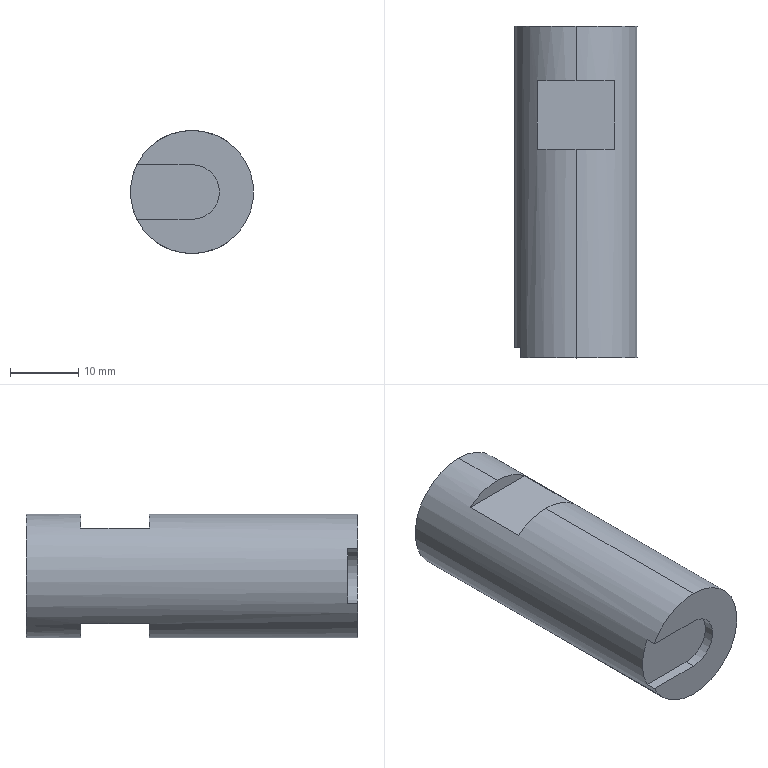Part | STEP file | OP10-150_clamp rod (L) | 1 solid | 18 faces | box 18 x 48.5 x 18 mm | volume 11527 mm3 | plane 11 | cylinder 5 | cone 2 | commonest cylinder face diameters 5 x2 18 x2 8 x1
STEP:
#1=CARTESIAN_POINT('',(0.,0.,0.));
#2=DIRECTION('',(0.,0.,1.));
#3=DIRECTION('',(1.,0.,0.));
#4=AXIS2_PLACEMENT_3D('',#1,#2,#3);
#5=CARTESIAN_POINT('',(0.,30.5,2.5));
#6=VERTEX_POINT('',#5);
#7=CARTESIAN_POINT('',(0.,48.5,2.5));
#8=VERTEX_POINT('',#7);
#9=CARTESIAN_POINT('',(0.,48.5,2.5));
#10=DIRECTION('',(0.,1.,0.));
#11=VECTOR('',#10,1.);
#12=LINE('',#9,#11);
#13=CARTESIAN_POINT('',(0.,48.5,0.));
#14=DIRECTION('',(0.,1.,0.));
#15=DIRECTION('',(0.,0.,1.));
#16=AXIS2_PLACEMENT_3D('',#13,#14,#15);
#17=CYLINDRICAL_SURFACE('',#16,2.5);
#18=CARTESIAN_POINT('',(6.283,0.));
#19=DIRECTION('',(0.,1.));
#20=VECTOR('',#19,1.);
#21=LINE('',#18,#20);
#22=(GEOMETRIC_REPRESENTATION_CONTEXT(2)PARAMETRIC_REPRESENTATION_CONTEXT()REPRESENTATION_CONTEXT('',''));
#23=DEFINITIONAL_REPRESENTATION('',(#21),#22);
#24=PCURVE('',#17,#23);
#25=CARTESIAN_POINT('',(0.,48.5,0.));
#26=DIRECTION('',(0.,1.,0.));
#27=DIRECTION('',(0.,0.,1.));
#28=AXIS2_PLACEMENT_3D('',#25,#26,#27);
#29=CYLINDRICAL_SURFACE('',#28,2.5);
#30=CARTESIAN_POINT('',(0.,0.));
#31=DIRECTION('',(0.,1.));
#32=VECTOR('',#31,1.);
#33=LINE('',#30,#32);
#34=(GEOMETRIC_REPRESENTATION_CONTEXT(2)PARAMETRIC_REPRESENTATION_CONTEXT()REPRESENTATION_CONTEXT('',''));
#35=DEFINITIONAL_REPRESENTATION('',(#33),#34);
#36=PCURVE('',#29,#35);
#37=SURFACE_CURVE('',#12,(#24,#36),.PCURVE_S1.);
#38=EDGE_CURVE('',#6,#8,#37,.T.);
#39=ORIENTED_EDGE('',*,*,#38,.T.);
#40=CARTESIAN_POINT('',(0.,48.5,-2.5));
#41=VERTEX_POINT('',#40);
#42=CARTESIAN_POINT('',(0.,48.5,0.));
#43=DIRECTION('',(0.,1.,0.));
#44=DIRECTION('',(0.,0.,1.));
#45=AXIS2_PLACEMENT_3D('',#42,#43,#44);
#46=CIRCLE('',#45,2.5);
#47=CARTESIAN_POINT('',(0.,0.));
#48=DIRECTION('',(1.,0.));
#49=VECTOR('',#48,1.);
#50=LINE('',#47,#49);
#51=(GEOMETRIC_REPRESENTATION_CONTEXT(2)PARAMETRIC_REPRESENTATION_CONTEXT()REPRESENTATION_CONTEXT('',''));
#52=DEFINITIONAL_REPRESENTATION('',(#50),#51);
#53=PCURVE('',#17,#52);
#54=CARTESIAN_POINT('',(0.,48.5,0.));
#55=DIRECTION('',(0.,1.,0.));
#56=DIRECTION('',(0.,0.,1.));
#57=AXIS2_PLACEMENT_3D('',#54,#55,#56);
#58=PLANE('',#57);
#59=CARTESIAN_POINT('',(0.,0.));
#60=DIRECTION('',(1.,0.));
#61=AXIS2_PLACEMENT_2D('',#59,#60);
#62=CIRCLE('',#61,2.5);
#63=(GEOMETRIC_REPRESENTATION_CONTEXT(2)PARAMETRIC_REPRESENTATION_CONTEXT()REPRESENTATION_CONTEXT('',''));
#64=DEFINITIONAL_REPRESENTATION('',(#62),#63);
#65=PCURVE('',#58,#64);
#66=SURFACE_CURVE('',#46,(#53,#65),.PCURVE_S1.);
#67=EDGE_CURVE('',#41,#8,#66,.T.);
#68=ORIENTED_EDGE('',*,*,#67,.F.);
#69=CARTESIAN_POINT('',(0.,30.5,-2.5));
#70=VERTEX_POINT('',#69);
#71=CARTESIAN_POINT('',(0.,48.5,-2.5));
#72=DIRECTION('',(0.,1.,0.));
#73=VECTOR('',#72,1.);
#74=LINE('',#71,#73);
#75=CARTESIAN_POINT('',(3.142,0.));
#76=DIRECTION('',(0.,1.));
#77=VECTOR('',#76,1.);
#78=LINE('',#75,#77);
#79=(GEOMETRIC_REPRESENTATION_CONTEXT(2)PARAMETRIC_REPRESENTATION_CONTEXT()REPRESENTATION_CONTEXT('',''));
#80=DEFINITIONAL_REPRESENTATION('',(#78),#79);
#81=PCURVE('',#17,#80);
#82=CARTESIAN_POINT('',(3.142,0.));
#83=DIRECTION('',(0.,1.));
#84=VECTOR('',#83,1.);
#85=LINE('',#82,#84);
#86=(GEOMETRIC_REPRESENTATION_CONTEXT(2)PARAMETRIC_REPRESENTATION_CONTEXT()REPRESENTATION_CONTEXT('',''));
#87=DEFINITIONAL_REPRESENTATION('',(#85),#86);
#88=PCURVE('',#29,#87);
#89=SURFACE_CURVE('',#74,(#81,#88),.PCURVE_S1.);
#90=EDGE_CURVE('',#70,#41,#89,.T.);
#91=ORIENTED_EDGE('',*,*,#90,.F.);
#92=CARTESIAN_POINT('',(0.,30.5,0.));
#93=DIRECTION('',(0.,1.,0.));
#94=DIRECTION('',(0.,0.,1.));
#95=AXIS2_PLACEMENT_3D('',#92,#93,#94);
#96=CIRCLE('',#95,2.5);
#97=CARTESIAN_POINT('',(0.,-18.));
#98=DIRECTION('',(1.,0.));
#99=VECTOR('',#98,1.);
#100=LINE('',#97,#99);
#101=(GEOMETRIC_REPRESENTATION_CONTEXT(2)PARAMETRIC_REPRESENTATION_CONTEXT()REPRESENTATION_CONTEXT('',''));
#102=DEFINITIONAL_REPRESENTATION('',(#100),#101);
#103=PCURVE('',#17,#102);
#104=CARTESIAN_POINT('',(0.,30.5,0.));
#105=DIRECTION('',(0.,1.,0.));
#106=DIRECTION('',(0.,0.,1.));
#107=AXIS2_PLACEMENT_3D('',#104,#105,#106);
#108=CONICAL_SURFACE('',#107,2.5,1.03);
#109=CARTESIAN_POINT('',(0.,0.));
#110=DIRECTION('',(1.,0.));
#111=VECTOR('',#110,1.);
#112=LINE('',#109,#111);
#113=(GEOMETRIC_REPRESENTATION_CONTEXT(2)PARAMETRIC_REPRESENTATION_CONTEXT()REPRESENTATION_CONTEXT('',''));
#114=DEFINITIONAL_REPRESENTATION('',(#112),#113);
#115=PCURVE('',#108,#114);
#116=SURFACE_CURVE('',#96,(#103,#115),.PCURVE_S1.);
#117=EDGE_CURVE('',#70,#6,#116,.T.);
#118=ORIENTED_EDGE('',*,*,#117,.T.);
#119=EDGE_LOOP('',(#39,#68,#91,#118));
#120=FACE_BOUND('',#119,.F.);
#121=ADVANCED_FACE('',(#120),#17,.F.);
#122=ORIENTED_EDGE('',*,*,#117,.F.);
#123=CARTESIAN_POINT('',(0.,28.998,0.));
#124=VERTEX_POINT('',#123);
#125=CARTESIAN_POINT('',(0.,30.5,-2.5));
#126=DIRECTION('',(0.,0.515,-0.8572));
#127=VECTOR('',#126,1.);
#128=LINE('',#125,#127);
#129=CARTESIAN_POINT('',(3.142,0.));
#130=DIRECTION('',(0.,1.));
#131=VECTOR('',#130,1.);
#132=LINE('',#129,#131);
#133=(GEOMETRIC_REPRESENTATION_CONTEXT(2)PARAMETRIC_REPRESENTATION_CONTEXT()REPRESENTATION_CONTEXT('',''));
#134=DEFINITIONAL_REPRESENTATION('',(#132),#133);
#135=PCURVE('',#108,#134);
#136=CARTESIAN_POINT('',(0.,30.5,0.));
#137=DIRECTION('',(0.,1.,0.));
#138=DIRECTION('',(0.,0.,1.));
#139=AXIS2_PLACEMENT_3D('',#136,#137,#138);
#140=CONICAL_SURFACE('',#139,2.5,1.03);
#141=CARTESIAN_POINT('',(3.142,0.));
#142=DIRECTION('',(0.,1.));
#143=VECTOR('',#142,1.);
#144=LINE('',#141,#143);
#145=(GEOMETRIC_REPRESENTATION_CONTEXT(2)PARAMETRIC_REPRESENTATION_CONTEXT()REPRESENTATION_CONTEXT('',''));
#146=DEFINITIONAL_REPRESENTATION('',(#144),#145);
#147=PCURVE('',#140,#146);
#148=SURFACE_CURVE('',#128,(#135,#147),.PCURVE_S1.);
#149=EDGE_CURVE('',#124,#70,#148,.T.);
#150=ORIENTED_EDGE('',*,*,#149,.F.);
#151=CARTESIAN_POINT('',(0.,30.5,2.5));
#152=DIRECTION('',(0.,0.515,0.8572));
#153=VECTOR('',#152,1.);
#154=LINE('',#151,#153);
#155=CARTESIAN_POINT('',(6.283,0.));
#156=DIRECTION('',(0.,1.));
#157=VECTOR('',#156,1.);
#158=LINE('',#155,#157);
#159=(GEOMETRIC_REPRESENTATION_CONTEXT(2)PARAMETRIC_REPRESENTATION_CONTEXT()REPRESENTATION_CONTEXT('',''));
#160=DEFINITIONAL_REPRESENTATION('',(#158),#159);
#161=PCURVE('',#108,#160);
#162=CARTESIAN_POINT('',(0.,0.));
#163=DIRECTION('',(0.,1.));
#164=VECTOR('',#163,1.);
#165=LINE('',#162,#164);
#166=(GEOMETRIC_REPRESENTATION_CONTEXT(2)PARAMETRIC_REPRESENTATION_CONTEXT()REPRESENTATION_CONTEXT('',''));
#167=DEFINITIONAL_REPRESENTATION('',(#165),#166);
#168=PCURVE('',#140,#167);
#169=SURFACE_CURVE('',#154,(#161,#168),.PCURVE_S1.);
#170=EDGE_CURVE('',#124,#6,#169,.T.);
#171=ORIENTED_EDGE('',*,*,#170,.T.);
#172=EDGE_LOOP('',(#122,#150,#171));
#173=FACE_BOUND('',#172,.F.);
#174=ADVANCED_FACE('',(#173),#108,.F.);
#175=CARTESIAN_POINT('',(0.,48.5,9.));
#176=VERTEX_POINT('',#175);
#177=CARTESIAN_POINT('',(0.,48.5,-9.));
#178=VERTEX_POINT('',#177);
#179=CARTESIAN_POINT('',(0.,48.5,0.));
#180=DIRECTION('',(0.,1.,0.));
#181=DIRECTION('',(0.,0.,1.));
#182=AXIS2_PLACEMENT_3D('',#179,#180,#181);
#183=CIRCLE('',#182,9.);
#184=CARTESIAN_POINT('',(0.,48.5,0.));
#185=DIRECTION('',(0.,-1.,0.));
#186=DIRECTION('',(0.,0.,-1.));
#187=AXIS2_PLACEMENT_3D('',#184,#185,#186);
#188=CYLINDRICAL_SURFACE('',#187,9.);
#189=CARTESIAN_POINT('',(3.142,0.));
#190=DIRECTION('',(-1.,0.));
#191=VECTOR('',#190,1.);
#192=LINE('',#189,#191);
#193=(GEOMETRIC_REPRESENTATION_CONTEXT(2)PARAMETRIC_REPRESENTATION_CONTEXT()REPRESENTATION_CONTEXT('',''));
#194=DEFINITIONAL_REPRESENTATION('',(#192),#193);
#195=PCURVE('',#188,#194);
#196=CARTESIAN_POINT('',(0.,0.));
#197=DIRECTION('',(1.,0.));
#198=AXIS2_PLACEMENT_2D('',#196,#197);
#199=CIRCLE('',#198,9.);
#200=(GEOMETRIC_REPRESENTATION_CONTEXT(2)PARAMETRIC_REPRESENTATION_CONTEXT()REPRESENTATION_CONTEXT('',''));
#201=DEFINITIONAL_REPRESENTATION('',(#199),#200);
#202=PCURVE('',#58,#201);
#203=SURFACE_CURVE('',#183,(#195,#202),.PCURVE_S1.);
#204=EDGE_CURVE('',#176,#178,#203,.T.);
#205=ORIENTED_EDGE('',*,*,#204,.F.);
#206=CARTESIAN_POINT('',(0.,40.5,9.));
#207=VERTEX_POINT('',#206);
#208=CARTESIAN_POINT('',(0.,48.5,9.));
#209=DIRECTION('',(0.,-1.,0.));
#210=VECTOR('',#209,1.);
#211=LINE('',#208,#210);
#212=CARTESIAN_POINT('',(3.142,0.));
#213=DIRECTION('',(0.,1.));
#214=VECTOR('',#213,1.);
#215=LINE('',#212,#214);
#216=(GEOMETRIC_REPRESENTATION_CONTEXT(2)PARAMETRIC_REPRESENTATION_CONTEXT()REPRESENTATION_CONTEXT('',''));
#217=DEFINITIONAL_REPRESENTATION('',(#215),#216);
#218=PCURVE('',#188,#217);
#219=CARTESIAN_POINT('',(0.,48.5,0.));
#220=DIRECTION('',(0.,-1.,0.));
#221=DIRECTION('',(0.,0.,-1.));
#222=AXIS2_PLACEMENT_3D('',#219,#220,#221);
#223=CYLINDRICAL_SURFACE('',#222,9.);
#224=CARTESIAN_POINT('',(3.142,0.));
#225=DIRECTION('',(0.,1.));
#226=VECTOR('',#225,1.);
#227=LINE('',#224,#226);
#228=(GEOMETRIC_REPRESENTATION_CONTEXT(2)PARAMETRIC_REPRESENTATION_CONTEXT()REPRESENTATION_CONTEXT('',''));
#229=DEFINITIONAL_REPRESENTATION('',(#227),#228);
#230=PCURVE('',#223,#229);
#231=SURFACE_CURVE('',#211,(#218,#230),.PCURVE_S1.);
#232=EDGE_CURVE('',#176,#207,#231,.T.);
#233=ORIENTED_EDGE('',*,*,#232,.T.);
#234=CARTESIAN_POINT('',(5.657,40.5,7.));
#235=VERTEX_POINT('',#234);
#236=CARTESIAN_POINT('',(0.,40.5,0.));
#237=DIRECTION('',(0.,-1.,0.));
#238=DIRECTION('',(0.,0.,-1.));
#239=AXIS2_PLACEMENT_3D('',#236,#237,#238);
#240=CIRCLE('',#239,9.);
#241=CARTESIAN_POINT('',(0.,8.));
#242=DIRECTION('',(1.,0.));
#243=VECTOR('',#242,1.);
#244=LINE('',#241,#243);
#245=(GEOMETRIC_REPRESENTATION_CONTEXT(2)PARAMETRIC_REPRESENTATION_CONTEXT()REPRESENTATION_CONTEXT('',''));
#246=DEFINITIONAL_REPRESENTATION('',(#244),#245);
#247=PCURVE('',#188,#246);
#248=CARTESIAN_POINT('',(-16.827,40.5,55.5));
#249=DIRECTION('',(0.,-1.,0.));
#250=DIRECTION('',(0.,0.,-1.));
#251=AXIS2_PLACEMENT_3D('',#248,#249,#250);
#252=PLANE('',#251);
#253=CARTESIAN_POINT('',(55.5,16.827));
#254=DIRECTION('',(1.,0.));
#255=AXIS2_PLACEMENT_2D('',#253,#254);
#256=CIRCLE('',#255,9.);
#257=(GEOMETRIC_REPRESENTATION_CONTEXT(2)PARAMETRIC_REPRESENTATION_CONTEXT()REPRESENTATION_CONTEXT('',''));
#258=DEFINITIONAL_REPRESENTATION('',(#256),#257);
#259=PCURVE('',#252,#258);
#260=SURFACE_CURVE('',#240,(#247,#259),.PCURVE_S1.);
#261=EDGE_CURVE('',#235,#207,#260,.T.);
#262=ORIENTED_EDGE('',*,*,#261,.F.);
#263=CARTESIAN_POINT('',(5.657,30.5,7.));
#264=VERTEX_POINT('',#263);
#265=CARTESIAN_POINT('',(5.657,48.5,7.));
#266=DIRECTION('',(0.,-1.,0.));
#267=VECTOR('',#266,1.);
#268=LINE('',#265,#267);
#269=CARTESIAN_POINT('',(2.462,0.));
#270=DIRECTION('',(0.,1.));
#271=VECTOR('',#270,1.);
#272=LINE('',#269,#271);
#273=(GEOMETRIC_REPRESENTATION_CONTEXT(2)PARAMETRIC_REPRESENTATION_CONTEXT()REPRESENTATION_CONTEXT('',''));
#274=DEFINITIONAL_REPRESENTATION('',(#272),#273);
#275=PCURVE('',#188,#274);
#276=CARTESIAN_POINT('',(0.,0.,7.));
#277=DIRECTION('',(0.,0.,-1.));
#278=DIRECTION('',(1.,0.,0.));
#279=AXIS2_PLACEMENT_3D('',#276,#277,#278);
#280=PLANE('',#279);
#281=CARTESIAN_POINT('',(5.657,-48.5));
#282=DIRECTION('',(0.,1.));
#283=VECTOR('',#282,1.);
#284=LINE('',#281,#283);
#285=(GEOMETRIC_REPRESENTATION_CONTEXT(2)PARAMETRIC_REPRESENTATION_CONTEXT()REPRESENTATION_CONTEXT('',''));
#286=DEFINITIONAL_REPRESENTATION('',(#284),#285);
#287=PCURVE('',#280,#286);
#288=SURFACE_CURVE('',#268,(#275,#287),.PCURVE_S1.);
#289=EDGE_CURVE('',#235,#264,#288,.T.);
#290=ORIENTED_EDGE('',*,*,#289,.T.);
#291=CARTESIAN_POINT('',(0.,30.5,9.));
#292=VERTEX_POINT('',#291);
#293=CARTESIAN_POINT('',(0.,30.5,0.));
#294=DIRECTION('',(0.,1.,0.));
#295=DIRECTION('',(0.,0.,1.));
#296=AXIS2_PLACEMENT_3D('',#293,#294,#295);
#297=CIRCLE('',#296,9.);
#298=CARTESIAN_POINT('',(3.142,18.));
#299=DIRECTION('',(-1.,0.));
#300=VECTOR('',#299,1.);
#301=LINE('',#298,#300);
#302=(GEOMETRIC_REPRESENTATION_CONTEXT(2)PARAMETRIC_REPRESENTATION_CONTEXT()REPRESENTATION_CONTEXT('',''));
#303=DEFINITIONAL_REPRESENTATION('',(#301),#302);
#304=PCURVE('',#188,#303);
#305=CARTESIAN_POINT('',(-16.827,30.5,55.5));
#306=DIRECTION('',(0.,1.,0.));
#307=DIRECTION('',(0.,0.,1.));
#308=AXIS2_PLACEMENT_3D('',#305,#306,#307);
#309=PLANE('',#308);
#310=CARTESIAN_POINT('',(-55.5,16.827));
#311=DIRECTION('',(1.,0.));
#312=AXIS2_PLACEMENT_2D('',#310,#311);
#313=CIRCLE('',#312,9.);
#314=(GEOMETRIC_REPRESENTATION_CONTEXT(2)PARAMETRIC_REPRESENTATION_CONTEXT()REPRESENTATION_CONTEXT('',''));
#315=DEFINITIONAL_REPRESENTATION('',(#313),#314);
#316=PCURVE('',#309,#315);
#317=SURFACE_CURVE('',#297,(#304,#316),.PCURVE_S1.);
#318=EDGE_CURVE('',#292,#264,#317,.T.);
#319=ORIENTED_EDGE('',*,*,#318,.F.);
#320=CARTESIAN_POINT('',(0.,0.,9.));
#321=VERTEX_POINT('',#320);
#322=CARTESIAN_POINT('',(0.,48.5,9.));
#323=DIRECTION('',(0.,-1.,0.));
#324=VECTOR('',#323,1.);
#325=LINE('',#322,#324);
#326=CARTESIAN_POINT('',(3.142,0.));
#327=DIRECTION('',(0.,1.));
#328=VECTOR('',#327,1.);
#329=LINE('',#326,#328);
#330=(GEOMETRIC_REPRESENTATION_CONTEXT(2)PARAMETRIC_REPRESENTATION_CONTEXT()REPRESENTATION_CONTEXT('',''));
#331=DEFINITIONAL_REPRESENTATION('',(#329),#330);
#332=PCURVE('',#188,#331);
#333=CARTESIAN_POINT('',(3.142,0.));
#334=DIRECTION('',(0.,1.));
#335=VECTOR('',#334,1.);
#336=LINE('',#333,#335);
#337=(GEOMETRIC_REPRESENTATION_CONTEXT(2)PARAMETRIC_REPRESENTATION_CONTEXT()REPRESENTATION_CONTEXT('',''));
#338=DEFINITIONAL_REPRESENTATION('',(#336),#337);
#339=PCURVE('',#223,#338);
#340=SURFACE_CURVE('',#325,(#332,#339),.PCURVE_S1.);
#341=EDGE_CURVE('',#292,#321,#340,.T.);
#342=ORIENTED_EDGE('',*,*,#341,.T.);
#343=CARTESIAN_POINT('',(0.,0.,-9.));
#344=VERTEX_POINT('',#343);
#345=CARTESIAN_POINT('',(0.,0.,0.));
#346=DIRECTION('',(0.,1.,0.));
#347=DIRECTION('',(0.,0.,1.));
#348=AXIS2_PLACEMENT_3D('',#345,#346,#347);
#349=CIRCLE('',#348,9.);
#350=CARTESIAN_POINT('',(3.142,48.5));
#351=DIRECTION('',(-1.,0.));
#352=VECTOR('',#351,1.);
#353=LINE('',#350,#352);
#354=(GEOMETRIC_REPRESENTATION_CONTEXT(2)PARAMETRIC_REPRESENTATION_CONTEXT()REPRESENTATION_CONTEXT('',''));
#355=DEFINITIONAL_REPRESENTATION('',(#353),#354);
#356=PCURVE('',#188,#355);
#357=CARTESIAN_POINT('',(0.,0.,0.));
#358=DIRECTION('',(0.,1.,0.));
#359=DIRECTION('',(0.,0.,1.));
#360=AXIS2_PLACEMENT_3D('',#357,#358,#359);
#361=PLANE('',#360);
#362=CARTESIAN_POINT('',(0.,0.));
#363=DIRECTION('',(1.,0.));
#364=AXIS2_PLACEMENT_2D('',#362,#363);
#365=CIRCLE('',#364,9.);
#366=(GEOMETRIC_REPRESENTATION_CONTEXT(2)PARAMETRIC_REPRESENTATION_CONTEXT()REPRESENTATION_CONTEXT('',''));
#367=DEFINITIONAL_REPRESENTATION('',(#365),#366);
#368=PCURVE('',#361,#367);
#369=SURFACE_CURVE('',#349,(#356,#368),.PCURVE_S1.);
#370=EDGE_CURVE('',#321,#344,#369,.T.);
#371=ORIENTED_EDGE('',*,*,#370,.T.);
#372=CARTESIAN_POINT('',(0.,30.5,-9.));
#373=VERTEX_POINT('',#372);
#374=CARTESIAN_POINT('',(0.,48.5,-9.));
#375=DIRECTION('',(0.,-1.,0.));
#376=VECTOR('',#375,1.);
#377=LINE('',#374,#376);
#378=CARTESIAN_POINT('',(0.,0.));
#379=DIRECTION('',(0.,1.));
#380=VECTOR('',#379,1.);
#381=LINE('',#378,#380);
#382=(GEOMETRIC_REPRESENTATION_CONTEXT(2)PARAMETRIC_REPRESENTATION_CONTEXT()REPRESENTATION_CONTEXT('',''));
#383=DEFINITIONAL_REPRESENTATION('',(#381),#382);
#384=PCURVE('',#188,#383);
#385=CARTESIAN_POINT('',(6.283,0.));
#386=DIRECTION('',(0.,1.));
#387=VECTOR('',#386,1.);
#388=LINE('',#385,#387);
#389=(GEOMETRIC_REPRESENTATION_CONTEXT(2)PARAMETRIC_REPRESENTATION_CONTEXT()REPRESENTATION_CONTEXT('',''));
#390=DEFINITIONAL_REPRESENTATION('',(#388),#389);
#391=PCURVE('',#223,#390);
#392=SURFACE_CURVE('',#377,(#384,#391),.PCURVE_S1.);
#393=EDGE_CURVE('',#373,#344,#392,.T.);
#394=ORIENTED_EDGE('',*,*,#393,.F.);
#395=CARTESIAN_POINT('',(5.657,30.5,-7.));
#396=VERTEX_POINT('',#395);
#397=CARTESIAN_POINT('',(0.,30.5,0.));
#398=DIRECTION('',(0.,-1.,0.));
#399=DIRECTION('',(0.,0.,-1.));
#400=AXIS2_PLACEMENT_3D('',#397,#398,#399);
#401=CIRCLE('',#400,9.);
#402=CARTESIAN_POINT('',(0.,18.));
#403=DIRECTION('',(1.,0.));
#404=VECTOR('',#403,1.);
#405=LINE('',#402,#404);
#406=(GEOMETRIC_REPRESENTATION_CONTEXT(2)PARAMETRIC_REPRESENTATION_CONTEXT()REPRESENTATION_CONTEXT('',''));
#407=DEFINITIONAL_REPRESENTATION('',(#405),#406);
#408=PCURVE('',#188,#407);
#409=CARTESIAN_POINT('',(-16.827,30.5,-55.5));
#410=DIRECTION('',(0.,-1.,0.));
#411=DIRECTION('',(0.,0.,-1.));
#412=AXIS2_PLACEMENT_3D('',#409,#410,#411);
#413=PLANE('',#412);
#414=CARTESIAN_POINT('',(-55.5,16.827));
#415=DIRECTION('',(1.,0.));
#416=AXIS2_PLACEMENT_2D('',#414,#415);
#417=CIRCLE('',#416,9.);
#418=(GEOMETRIC_REPRESENTATION_CONTEXT(2)PARAMETRIC_REPRESENTATION_CONTEXT()REPRESENTATION_CONTEXT('',''));
#419=DEFINITIONAL_REPRESENTATION('',(#417),#418);
#420=PCURVE('',#413,#419);
#421=SURFACE_CURVE('',#401,(#408,#420),.PCURVE_S1.);
#422=EDGE_CURVE('',#373,#396,#421,.T.);
#423=ORIENTED_EDGE('',*,*,#422,.T.);
#424=CARTESIAN_POINT('',(5.657,40.5,-7.));
#425=VERTEX_POINT('',#424);
#426=CARTESIAN_POINT('',(5.657,48.5,-7.));
#427=DIRECTION('',(0.,1.,0.));
#428=VECTOR('',#427,1.);
#429=LINE('',#426,#428);
#430=CARTESIAN_POINT('',(0.6797,0.));
#431=DIRECTION('',(0.,-1.));
#432=VECTOR('',#431,1.);
#433=LINE('',#430,#432);
#434=(GEOMETRIC_REPRESENTATION_CONTEXT(2)PARAMETRIC_REPRESENTATION_CONTEXT()REPRESENTATION_CONTEXT('',''));
#435=DEFINITIONAL_REPRESENTATION('',(#433),#434);
#436=PCURVE('',#188,#435);
#437=CARTESIAN_POINT('',(0.,0.,-7.));
#438=DIRECTION('',(0.,0.,1.));
#439=DIRECTION('',(1.,0.,0.));
#440=AXIS2_PLACEMENT_3D('',#437,#438,#439);
#441=PLANE('',#440);
#442=CARTESIAN_POINT('',(5.657,48.5));
#443=DIRECTION('',(0.,1.));
#444=VECTOR('',#443,1.);
#445=LINE('',#442,#444);
#446=(GEOMETRIC_REPRESENTATION_CONTEXT(2)PARAMETRIC_REPRESENTATION_CONTEXT()REPRESENTATION_CONTEXT('',''));
#447=DEFINITIONAL_REPRESENTATION('',(#445),#446);
#448=PCURVE('',#441,#447);
#449=SURFACE_CURVE('',#429,(#436,#448),.PCURVE_S1.);
#450=EDGE_CURVE('',#396,#425,#449,.T.);
#451=ORIENTED_EDGE('',*,*,#450,.T.);
#452=CARTESIAN_POINT('',(0.,40.5,-9.));
#453=VERTEX_POINT('',#452);
#454=CARTESIAN_POINT('',(0.,40.5,0.));
#455=DIRECTION('',(0.,1.,0.));
#456=DIRECTION('',(0.,0.,1.));
#457=AXIS2_PLACEMENT_3D('',#454,#455,#456);
#458=CIRCLE('',#457,9.);
#459=CARTESIAN_POINT('',(3.142,8.));
#460=DIRECTION('',(-1.,0.));
#461=VECTOR('',#460,1.);
#462=LINE('',#459,#461);
#463=(GEOMETRIC_REPRESENTATION_CONTEXT(2)PARAMETRIC_REPRESENTATION_CONTEXT()REPRESENTATION_CONTEXT('',''));
#464=DEFINITIONAL_REPRESENTATION('',(#462),#463);
#465=PCURVE('',#188,#464);
#466=CARTESIAN_POINT('',(-16.827,40.5,-55.5));
#467=DIRECTION('',(0.,1.,0.));
#468=DIRECTION('',(0.,0.,1.));
#469=AXIS2_PLACEMENT_3D('',#466,#467,#468);
#470=PLANE('',#469);
#471=CARTESIAN_POINT('',(55.5,16.827));
#472=DIRECTION('',(1.,0.));
#473=AXIS2_PLACEMENT_2D('',#471,#472);
#474=CIRCLE('',#473,9.);
#475=(GEOMETRIC_REPRESENTATION_CONTEXT(2)PARAMETRIC_REPRESENTATION_CONTEXT()REPRESENTATION_CONTEXT('',''));
#476=DEFINITIONAL_REPRESENTATION('',(#474),#475);
#477=PCURVE('',#470,#476);
#478=SURFACE_CURVE('',#458,(#465,#477),.PCURVE_S1.);
#479=EDGE_CURVE('',#425,#453,#478,.T.);
#480=ORIENTED_EDGE('',*,*,#479,.T.);
#481=CARTESIAN_POINT('',(0.,48.5,-9.));
#482=DIRECTION('',(0.,-1.,0.));
#483=VECTOR('',#482,1.);
#484=LINE('',#481,#483);
#485=CARTESIAN_POINT('',(0.,0.));
#486=DIRECTION('',(0.,1.));
#487=VECTOR('',#486,1.);
#488=LINE('',#485,#487);
#489=(GEOMETRIC_REPRESENTATION_CONTEXT(2)PARAMETRIC_REPRESENTATION_CONTEXT()REPRESENTATION_CONTEXT('',''));
#490=DEFINITIONAL_REPRESENTATION('',(#488),#489);
#491=PCURVE('',#188,#490);
#492=CARTESIAN_POINT('',(6.283,0.));
#493=DIRECTION('',(0.,1.));
#494=VECTOR('',#493,1.);
#495=LINE('',#492,#494);
#496=(GEOMETRIC_REPRESENTATION_CONTEXT(2)PARAMETRIC_REPRESENTATION_CONTEXT()REPRESENTATION_CONTEXT('',''));
#497=DEFINITIONAL_REPRESENTATION('',(#495),#496);
#498=PCURVE('',#223,#497);
#499=SURFACE_CURVE('',#484,(#491,#498),.PCURVE_S1.);
#500=EDGE_CURVE('',#178,#453,#499,.T.);
#501=ORIENTED_EDGE('',*,*,#500,.F.);
#502=EDGE_LOOP('',(#205,#233,#262,#290,#319,#342,#371,#394,#423,#451,#480,#501));
#503=FACE_BOUND('',#502,.T.);
#504=ADVANCED_FACE('',(#503),#188,.T.);
#505=ORIENTED_EDGE('',*,*,#232,.F.);
#506=CARTESIAN_POINT('',(0.,48.5,0.));
#507=DIRECTION('',(0.,1.,0.));
#508=DIRECTION('',(0.,0.,1.));
#509=AXIS2_PLACEMENT_3D('',#506,#507,#508);
#510=CIRCLE('',#509,9.);
#511=CARTESIAN_POINT('',(9.425,0.));
#512=DIRECTION('',(-1.,0.));
#513=VECTOR('',#512,1.);
#514=LINE('',#511,#513);
#515=(GEOMETRIC_REPRESENTATION_CONTEXT(2)PARAMETRIC_REPRESENTATION_CONTEXT()REPRESENTATION_CONTEXT('',''));
#516=DEFINITIONAL_REPRESENTATION('',(#514),#515);
#517=PCURVE('',#223,#516);
#518=CARTESIAN_POINT('',(0.,0.));
#519=DIRECTION('',(1.,0.));
#520=AXIS2_PLACEMENT_2D('',#518,#519);
#521=CIRCLE('',#520,9.);
#522=(GEOMETRIC_REPRESENTATION_CONTEXT(2)PARAMETRIC_REPRESENTATION_CONTEXT()REPRESENTATION_CONTEXT('',''));
#523=DEFINITIONAL_REPRESENTATION('',(#521),#522);
#524=PCURVE('',#58,#523);
#525=SURFACE_CURVE('',#510,(#517,#524),.PCURVE_S1.);
#526=EDGE_CURVE('',#178,#176,#525,.T.);
#527=ORIENTED_EDGE('',*,*,#526,.F.);
#528=ORIENTED_EDGE('',*,*,#500,.T.);
#529=CARTESIAN_POINT('',(-5.657,40.5,-7.));
#530=VERTEX_POINT('',#529);
#531=CARTESIAN_POINT('',(0.,40.5,0.));
#532=DIRECTION('',(0.,1.,0.));
#533=DIRECTION('',(0.,0.,1.));
#534=AXIS2_PLACEMENT_3D('',#531,#532,#533);
#535=CIRCLE('',#534,9.);
#536=CARTESIAN_POINT('',(9.425,8.));
#537=DIRECTION('',(-1.,0.));
#538=VECTOR('',#537,1.);
#539=LINE('',#536,#538);
#540=(GEOMETRIC_REPRESENTATION_CONTEXT(2)PARAMETRIC_REPRESENTATION_CONTEXT()REPRESENTATION_CONTEXT('',''));
#541=DEFINITIONAL_REPRESENTATION('',(#539),#540);
#542=PCURVE('',#223,#541);
#543=CARTESIAN_POINT('',(55.5,16.827));
#544=DIRECTION('',(1.,0.));
#545=AXIS2_PLACEMENT_2D('',#543,#544);
#546=CIRCLE('',#545,9.);
#547=(GEOMETRIC_REPRESENTATION_CONTEXT(2)PARAMETRIC_REPRESENTATION_CONTEXT()REPRESENTATION_CONTEXT('',''));
#548=DEFINITIONAL_REPRESENTATION('',(#546),#547);
#549=PCURVE('',#470,#548);
#550=SURFACE_CURVE('',#535,(#542,#549),.PCURVE_S1.);
#551=EDGE_CURVE('',#453,#530,#550,.T.);
#552=ORIENTED_EDGE('',*,*,#551,.T.);
#553=CARTESIAN_POINT('',(-5.657,30.5,-7.));
#554=VERTEX_POINT('',#553);
#555=CARTESIAN_POINT('',(-5.657,48.5,-7.));
#556=DIRECTION('',(0.,-1.,0.));
#557=VECTOR('',#556,1.);
#558=LINE('',#555,#557);
#559=CARTESIAN_POINT('',(5.604,0.));
#560=DIRECTION('',(0.,1.));
#561=VECTOR('',#560,1.);
#562=LINE('',#559,#561);
#563=(GEOMETRIC_REPRESENTATION_CONTEXT(2)PARAMETRIC_REPRESENTATION_CONTEXT()REPRESENTATION_CONTEXT('',''));
#564=DEFINITIONAL_REPRESENTATION('',(#562),#563);
#565=PCURVE('',#223,#564);
#566=CARTESIAN_POINT('',(-5.657,48.5));
#567=DIRECTION('',(0.,-1.));
#568=VECTOR('',#567,1.);
#569=LINE('',#566,#568);
#570=(GEOMETRIC_REPRESENTATION_CONTEXT(2)PARAMETRIC_REPRESENTATION_CONTEXT()REPRESENTATION_CONTEXT('',''));
#571=DEFINITIONAL_REPRESENTATION('',(#569),#570);
#572=PCURVE('',#441,#571);
#573=SURFACE_CURVE('',#558,(#565,#572),.PCURVE_S1.);
#574=EDGE_CURVE('',#530,#554,#573,.T.);
#575=ORIENTED_EDGE('',*,*,#574,.T.);
#576=CARTESIAN_POINT('',(0.,30.5,0.));
#577=DIRECTION('',(0.,-1.,0.));
#578=DIRECTION('',(0.,0.,-1.));
#579=AXIS2_PLACEMENT_3D('',#576,#577,#578);
#580=CIRCLE('',#579,9.);
#581=CARTESIAN_POINT('',(0.,18.));
#582=DIRECTION('',(1.,0.));
#583=VECTOR('',#582,1.);
#584=LINE('',#581,#583);
#585=(GEOMETRIC_REPRESENTATION_CONTEXT(2)PARAMETRIC_REPRESENTATION_CONTEXT()REPRESENTATION_CONTEXT('',''));
#586=DEFINITIONAL_REPRESENTATION('',(#584),#585);
#587=PCURVE('',#223,#586);
#588=CARTESIAN_POINT('',(-55.5,16.827));
#589=DIRECTION('',(1.,0.));
#590=AXIS2_PLACEMENT_2D('',#588,#589);
#591=CIRCLE('',#590,9.);
#592=(GEOMETRIC_REPRESENTATION_CONTEXT(2)PARAMETRIC_REPRESENTATION_CONTEXT()REPRESENTATION_CONTEXT('',''));
#593=DEFINITIONAL_REPRESENTATION('',(#591),#592);
#594=PCURVE('',#413,#593);
#595=SURFACE_CURVE('',#580,(#587,#594),.PCURVE_S1.);
#596=EDGE_CURVE('',#554,#373,#595,.T.);
#597=ORIENTED_EDGE('',*,*,#596,.T.);
#598=ORIENTED_EDGE('',*,*,#393,.T.);
#599=CARTESIAN_POINT('',(-8.062,0.,-4.));
#600=VERTEX_POINT('',#599);
#601=CARTESIAN_POINT('',(0.,0.,0.));
#602=DIRECTION('',(0.,1.,0.));
#603=DIRECTION('',(0.,0.,1.));
#604=AXIS2_PLACEMENT_3D('',#601,#602,#603);
#605=CIRCLE('',#604,9.);
#606=CARTESIAN_POINT('',(9.425,48.5));
#607=DIRECTION('',(-1.,0.));
#608=VECTOR('',#607,1.);
#609=LINE('',#606,#608);
#610=(GEOMETRIC_REPRESENTATION_CONTEXT(2)PARAMETRIC_REPRESENTATION_CONTEXT()REPRESENTATION_CONTEXT('',''));
#611=DEFINITIONAL_REPRESENTATION('',(#609),#610);
#612=PCURVE('',#223,#611);
#613=CARTESIAN_POINT('',(0.,0.));
#614=DIRECTION('',(1.,0.));
#615=AXIS2_PLACEMENT_2D('',#613,#614);
#616=CIRCLE('',#615,9.);
#617=(GEOMETRIC_REPRESENTATION_CONTEXT(2)PARAMETRIC_REPRESENTATION_CONTEXT()REPRESENTATION_CONTEXT('',''));
#618=DEFINITIONAL_REPRESENTATION('',(#616),#617);
#619=PCURVE('',#361,#618);
#620=SURFACE_CURVE('',#605,(#612,#619),.PCURVE_S1.);
#621=EDGE_CURVE('',#344,#600,#620,.T.);
#622=ORIENTED_EDGE('',*,*,#621,.T.);
#623=CARTESIAN_POINT('',(-8.062,1.5,-4.));
#624=VERTEX_POINT('',#623);
#625=CARTESIAN_POINT('',(-8.062,48.5,-4.));
#626=DIRECTION('',(0.,1.,0.));
#627=VECTOR('',#626,1.);
#628=LINE('',#625,#627);
#629=CARTESIAN_POINT('',(5.173,0.));
#630=DIRECTION('',(0.,-1.));
#631=VECTOR('',#630,1.);
#632=LINE('',#629,#631);
#633=(GEOMETRIC_REPRESENTATION_CONTEXT(2)PARAMETRIC_REPRESENTATION_CONTEXT()REPRESENTATION_CONTEXT('',''));
#634=DEFINITIONAL_REPRESENTATION('',(#632),#633);
#635=PCURVE('',#223,#634);
#636=CARTESIAN_POINT('',(-9.,1.5,-4.));
#637=DIRECTION('',(0.,0.,-1.));
#638=DIRECTION('',(-1.,0.,0.));
#639=AXIS2_PLACEMENT_3D('',#636,#637,#638);
#640=PLANE('',#639);
#641=CARTESIAN_POINT('',(-0.9377,47.));
#642=DIRECTION('',(0.,1.));
#643=VECTOR('',#642,1.);
#644=LINE('',#641,#643);
#645=(GEOMETRIC_REPRESENTATION_CONTEXT(2)PARAMETRIC_REPRESENTATION_CONTEXT()REPRESENTATION_CONTEXT('',''));
#646=DEFINITIONAL_REPRESENTATION('',(#644),#645);
#647=PCURVE('',#640,#646);
#648=SURFACE_CURVE('',#628,(#635,#647),.PCURVE_S1.);
#649=EDGE_CURVE('',#600,#624,#648,.T.);
#650=ORIENTED_EDGE('',*,*,#649,.T.);
#651=CARTESIAN_POINT('',(-8.062,1.5,4.));
#652=VERTEX_POINT('',#651);
#653=CARTESIAN_POINT('',(0.,1.5,0.));
#654=DIRECTION('',(0.,-1.,0.));
#655=DIRECTION('',(0.,0.,-1.));
#656=AXIS2_PLACEMENT_3D('',#653,#654,#655);
#657=CIRCLE('',#656,9.);
#658=CARTESIAN_POINT('',(0.,47.));
#659=DIRECTION('',(1.,0.));
#660=VECTOR('',#659,1.);
#661=LINE('',#658,#660);
#662=(GEOMETRIC_REPRESENTATION_CONTEXT(2)PARAMETRIC_REPRESENTATION_CONTEXT()REPRESENTATION_CONTEXT('',''));
#663=DEFINITIONAL_REPRESENTATION('',(#661),#662);
#664=PCURVE('',#223,#663);
#665=CARTESIAN_POINT('',(-9.,1.5,0.));
#666=DIRECTION('',(0.,-1.,0.));
#667=DIRECTION('',(0.,0.,-1.));
#668=AXIS2_PLACEMENT_3D('',#665,#666,#667);
#669=PLANE('',#668);
#670=CARTESIAN_POINT('',(0.,9.));
#671=DIRECTION('',(1.,0.));
#672=AXIS2_PLACEMENT_2D('',#670,#671);
#673=CIRCLE('',#672,9.);
#674=(GEOMETRIC_REPRESENTATION_CONTEXT(2)PARAMETRIC_REPRESENTATION_CONTEXT()REPRESENTATION_CONTEXT('',''));
#675=DEFINITIONAL_REPRESENTATION('',(#673),#674);
#676=PCURVE('',#669,#675);
#677=SURFACE_CURVE('',#657,(#664,#676),.PCURVE_S1.);
#678=EDGE_CURVE('',#652,#624,#677,.T.);
#679=ORIENTED_EDGE('',*,*,#678,.F.);
#680=CARTESIAN_POINT('',(-8.062,0.,4.));
#681=VERTEX_POINT('',#680);
#682=CARTESIAN_POINT('',(-8.062,48.5,4.));
#683=DIRECTION('',(0.,-1.,0.));
#684=VECTOR('',#683,1.);
#685=LINE('',#682,#684);
#686=CARTESIAN_POINT('',(4.252,0.));
#687=DIRECTION('',(0.,1.));
#688=VECTOR('',#687,1.);
#689=LINE('',#686,#688);
#690=(GEOMETRIC_REPRESENTATION_CONTEXT(2)PARAMETRIC_REPRESENTATION_CONTEXT()REPRESENTATION_CONTEXT('',''));
#691=DEFINITIONAL_REPRESENTATION('',(#689),#690);
#692=PCURVE('',#223,#691);
#693=CARTESIAN_POINT('',(-9.,1.5,4.));
#694=DIRECTION('',(0.,0.,1.));
#695=DIRECTION('',(1.,0.,0.));
#696=AXIS2_PLACEMENT_3D('',#693,#694,#695);
#697=PLANE('',#696);
#698=CARTESIAN_POINT('',(0.9377,47.));
#699=DIRECTION('',(0.,-1.));
#700=VECTOR('',#699,1.);
#701=LINE('',#698,#700);
#702=(GEOMETRIC_REPRESENTATION_CONTEXT(2)PARAMETRIC_REPRESENTATION_CONTEXT()REPRESENTATION_CONTEXT('',''));
#703=DEFINITIONAL_REPRESENTATION('',(#701),#702);
#704=PCURVE('',#697,#703);
#705=SURFACE_CURVE('',#685,(#692,#704),.PCURVE_S1.);
#706=EDGE_CURVE('',#652,#681,#705,.T.);
#707=ORIENTED_EDGE('',*,*,#706,.T.);
#708=CARTESIAN_POINT('',(0.,0.,0.));
#709=DIRECTION('',(0.,1.,0.));
#710=DIRECTION('',(0.,0.,1.));
#711=AXIS2_PLACEMENT_3D('',#708,#709,#710);
#712=CIRCLE('',#711,9.);
#713=CARTESIAN_POINT('',(9.425,48.5));
#714=DIRECTION('',(-1.,0.));
#715=VECTOR('',#714,1.);
#716=LINE('',#713,#715);
#717=(GEOMETRIC_REPRESENTATION_CONTEXT(2)PARAMETRIC_REPRESENTATION_CONTEXT()REPRESENTATION_CONTEXT('',''));
#718=DEFINITIONAL_REPRESENTATION('',(#716),#717);
#719=PCURVE('',#223,#718);
#720=CARTESIAN_POINT('',(0.,0.));
#721=DIRECTION('',(1.,0.));
#722=AXIS2_PLACEMENT_2D('',#720,#721);
#723=CIRCLE('',#722,9.);
#724=(GEOMETRIC_REPRESENTATION_CONTEXT(2)PARAMETRIC_REPRESENTATION_CONTEXT()REPRESENTATION_CONTEXT('',''));
#725=DEFINITIONAL_REPRESENTATION('',(#723),#724);
#726=PCURVE('',#361,#725);
#727=SURFACE_CURVE('',#712,(#719,#726),.PCURVE_S1.);
#728=EDGE_CURVE('',#681,#321,#727,.T.);
#729=ORIENTED_EDGE('',*,*,#728,.T.);
#730=ORIENTED_EDGE('',*,*,#341,.F.);
#731=CARTESIAN_POINT('',(-5.657,30.5,7.));
#732=VERTEX_POINT('',#731);
#733=CARTESIAN_POINT('',(0.,30.5,0.));
#734=DIRECTION('',(0.,1.,0.));
#735=DIRECTION('',(0.,0.,1.));
#736=AXIS2_PLACEMENT_3D('',#733,#734,#735);
#737=CIRCLE('',#736,9.);
#738=CARTESIAN_POINT('',(9.425,18.));
#739=DIRECTION('',(-1.,0.));
#740=VECTOR('',#739,1.);
#741=LINE('',#738,#740);
#742=(GEOMETRIC_REPRESENTATION_CONTEXT(2)PARAMETRIC_REPRESENTATION_CONTEXT()REPRESENTATION_CONTEXT('',''));
#743=DEFINITIONAL_REPRESENTATION('',(#741),#742);
#744=PCURVE('',#223,#743);
#745=CARTESIAN_POINT('',(-55.5,16.827));
#746=DIRECTION('',(1.,0.));
#747=AXIS2_PLACEMENT_2D('',#745,#746);
#748=CIRCLE('',#747,9.);
#749=(GEOMETRIC_REPRESENTATION_CONTEXT(2)PARAMETRIC_REPRESENTATION_CONTEXT()REPRESENTATION_CONTEXT('',''));
#750=DEFINITIONAL_REPRESENTATION('',(#748),#749);
#751=PCURVE('',#309,#750);
#752=SURFACE_CURVE('',#737,(#744,#751),.PCURVE_S1.);
#753=EDGE_CURVE('',#732,#292,#752,.T.);
#754=ORIENTED_EDGE('',*,*,#753,.F.);
#755=CARTESIAN_POINT('',(-5.657,40.5,7.));
#756=VERTEX_POINT('',#755);
#757=CARTESIAN_POINT('',(-5.657,48.5,7.));
#758=DIRECTION('',(0.,1.,0.));
#759=VECTOR('',#758,1.);
#760=LINE('',#757,#759);
#761=CARTESIAN_POINT('',(3.821,0.));
#762=DIRECTION('',(0.,-1.));
#763=VECTOR('',#762,1.);
#764=LINE('',#761,#763);
#765=(GEOMETRIC_REPRESENTATION_CONTEXT(2)PARAMETRIC_REPRESENTATION_CONTEXT()REPRESENTATION_CONTEXT('',''));
#766=DEFINITIONAL_REPRESENTATION('',(#764),#765);
#767=PCURVE('',#223,#766);
#768=CARTESIAN_POINT('',(-5.657,-48.5));
#769=DIRECTION('',(0.,-1.));
#770=VECTOR('',#769,1.);
#771=LINE('',#768,#770);
#772=(GEOMETRIC_REPRESENTATION_CONTEXT(2)PARAMETRIC_REPRESENTATION_CONTEXT()REPRESENTATION_CONTEXT('',''));
#773=DEFINITIONAL_REPRESENTATION('',(#771),#772);
#774=PCURVE('',#280,#773);
#775=SURFACE_CURVE('',#760,(#767,#774),.PCURVE_S1.);
#776=EDGE_CURVE('',#732,#756,#775,.T.);
#777=ORIENTED_EDGE('',*,*,#776,.T.);
#778=CARTESIAN_POINT('',(0.,40.5,0.));
#779=DIRECTION('',(0.,-1.,0.));
#780=DIRECTION('',(0.,0.,-1.));
#781=AXIS2_PLACEMENT_3D('',#778,#779,#780);
#782=CIRCLE('',#781,9.);
#783=CARTESIAN_POINT('',(0.,8.));
#784=DIRECTION('',(1.,0.));
#785=VECTOR('',#784,1.);
#786=LINE('',#783,#785);
#787=(GEOMETRIC_REPRESENTATION_CONTEXT(2)PARAMETRIC_REPRESENTATION_CONTEXT()REPRESENTATION_CONTEXT('',''));
#788=DEFINITIONAL_REPRESENTATION('',(#786),#787);
#789=PCURVE('',#223,#788);
#790=CARTESIAN_POINT('',(55.5,16.827));
#791=DIRECTION('',(1.,0.));
#792=AXIS2_PLACEMENT_2D('',#790,#791);
#793=CIRCLE('',#792,9.);
#794=(GEOMETRIC_REPRESENTATION_CONTEXT(2)PARAMETRIC_REPRESENTATION_CONTEXT()REPRESENTATION_CONTEXT('',''));
#795=DEFINITIONAL_REPRESENTATION('',(#793),#794);
#796=PCURVE('',#252,#795);
#797=SURFACE_CURVE('',#782,(#789,#796),.PCURVE_S1.);
#798=EDGE_CURVE('',#207,#756,#797,.T.);
#799=ORIENTED_EDGE('',*,*,#798,.F.);
#800=EDGE_LOOP('',(#505,#527,#528,#552,#575,#597,#598,#622,#650,#679,#707,#729,#730,#754,#777,#799));
#801=FACE_BOUND('',#800,.T.);
#802=ADVANCED_FACE('',(#801),#223,.T.);
#803=CARTESIAN_POINT('',(0.,48.5,0.));
#804=DIRECTION('',(0.,1.,0.));
#805=DIRECTION('',(0.,0.,1.));
#806=AXIS2_PLACEMENT_3D('',#803,#804,#805);
#807=CIRCLE('',#806,2.5);
#808=CARTESIAN_POINT('',(0.,0.));
#809=DIRECTION('',(1.,0.));
#810=AXIS2_PLACEMENT_2D('',#808,#809);
#811=CIRCLE('',#810,2.5);
#812=(GEOMETRIC_REPRESENTATION_CONTEXT(2)PARAMETRIC_REPRESENTATION_CONTEXT()REPRESENTATION_CONTEXT('',''));
#813=DEFINITIONAL_REPRESENTATION('',(#811),#812);
#814=PCURVE('',#58,#813);
#815=CARTESIAN_POINT('',(0.,0.));
#816=DIRECTION('',(1.,0.));
#817=VECTOR('',#816,1.);
#818=LINE('',#815,#817);
#819=(GEOMETRIC_REPRESENTATION_CONTEXT(2)PARAMETRIC_REPRESENTATION_CONTEXT()REPRESENTATION_CONTEXT('',''));
#820=DEFINITIONAL_REPRESENTATION('',(#818),#819);
#821=PCURVE('',#29,#820);
#822=SURFACE_CURVE('',#807,(#814,#821),.PCURVE_S1.);
#823=EDGE_CURVE('',#8,#41,#822,.T.);
#824=ORIENTED_EDGE('',*,*,#823,.F.);
#825=ORIENTED_EDGE('',*,*,#67,.F.);
#826=EDGE_LOOP('',(#824,#825));
#827=FACE_BOUND('',#826,.T.);
#828=ORIENTED_EDGE('',*,*,#526,.T.);
#829=ORIENTED_EDGE('',*,*,#204,.T.);
#830=EDGE_LOOP('',(#828,#829));
#831=FACE_BOUND('',#830,.T.);
#832=ADVANCED_FACE('',(#827,#831),#58,.T.);
#833=ORIENTED_EDGE('',*,*,#728,.F.);
#834=CARTESIAN_POINT('',(0.,0.,4.));
#835=VERTEX_POINT('',#834);
#836=CARTESIAN_POINT('',(-9.,0.,4.));
#837=DIRECTION('',(-1.,0.,0.));
#838=VECTOR('',#837,1.);
#839=LINE('',#836,#838);
#840=CARTESIAN_POINT('',(4.,-9.));
#841=DIRECTION('',(0.,-1.));
#842=VECTOR('',#841,1.);
#843=LINE('',#840,#842);
#844=(GEOMETRIC_REPRESENTATION_CONTEXT(2)PARAMETRIC_REPRESENTATION_CONTEXT()REPRESENTATION_CONTEXT('',''));
#845=DEFINITIONAL_REPRESENTATION('',(#843),#844);
#846=PCURVE('',#361,#845);
#847=CARTESIAN_POINT('',(0.,-1.5));
#848=DIRECTION('',(-1.,0.));
#849=VECTOR('',#848,1.);
#850=LINE('',#847,#849);
#851=(GEOMETRIC_REPRESENTATION_CONTEXT(2)PARAMETRIC_REPRESENTATION_CONTEXT()REPRESENTATION_CONTEXT('',''));
#852=DEFINITIONAL_REPRESENTATION('',(#850),#851);
#853=PCURVE('',#697,#852);
#854=SURFACE_CURVE('',#839,(#846,#853),.PCURVE_S1.);
#855=EDGE_CURVE('',#835,#681,#854,.T.);
#856=ORIENTED_EDGE('',*,*,#855,.F.);
#857=CARTESIAN_POINT('',(0.,0.,-4.));
#858=VERTEX_POINT('',#857);
#859=CARTESIAN_POINT('',(0.,0.,0.));
#860=DIRECTION('',(0.,-1.,0.));
#861=DIRECTION('',(0.,0.,-1.));
#862=AXIS2_PLACEMENT_3D('',#859,#860,#861);
#863=CIRCLE('',#862,4.);
#864=CARTESIAN_POINT('',(-4.,0.));
#865=CARTESIAN_POINT('',(-4.,6.928));
#866=CARTESIAN_POINT('',(2.,3.464));
#867=CARTESIAN_POINT('',(8.,0.));
#868=CARTESIAN_POINT('',(2.,-3.464));
#869=CARTESIAN_POINT('',(-4.,-6.928));
#870=CARTESIAN_POINT('',(-4.,0.));
#871=(BOUNDED_CURVE()B_SPLINE_CURVE(2,(#864,#865,#866,#867,#868,#869,#870),.UNSPECIFIED.,.T.,.F.)B_SPLINE_CURVE_WITH_KNOTS((1,2,2,2,2,1),(-2.094,0.,2.094,4.189,6.283,8.378),.UNSPECIFIED.)CURVE()GEOMETRIC_REPRESENTATION_ITEM()RATIONAL_B_SPLINE_CURVE((1.,0.5,1.,0.5,1.,0.5,1.))REPRESENTATION_ITEM(''));
#872=(GEOMETRIC_REPRESENTATION_CONTEXT(2)PARAMETRIC_REPRESENTATION_CONTEXT()REPRESENTATION_CONTEXT('',''));
#873=DEFINITIONAL_REPRESENTATION('',(#871),#872);
#874=PCURVE('',#361,#873);
#875=CARTESIAN_POINT('',(0.,1.5,0.));
#876=DIRECTION('',(0.,-1.,0.));
#877=DIRECTION('',(0.,0.,-1.));
#878=AXIS2_PLACEMENT_3D('',#875,#876,#877);
#879=CYLINDRICAL_SURFACE('',#878,4.);
#880=CARTESIAN_POINT('',(0.,1.5));
#881=DIRECTION('',(1.,0.));
#882=VECTOR('',#881,1.);
#883=LINE('',#880,#882);
#884=(GEOMETRIC_REPRESENTATION_CONTEXT(2)PARAMETRIC_REPRESENTATION_CONTEXT()REPRESENTATION_CONTEXT('',''));
#885=DEFINITIONAL_REPRESENTATION('',(#883),#884);
#886=PCURVE('',#879,#885);
#887=SURFACE_CURVE('',#863,(#874,#886),.PCURVE_S1.);
#888=EDGE_CURVE('',#858,#835,#887,.T.);
#889=ORIENTED_EDGE('',*,*,#888,.F.);
#890=CARTESIAN_POINT('',(0.,0.,-4.));
#891=DIRECTION('',(-1.,0.,0.));
#892=VECTOR('',#891,1.);
#893=LINE('',#890,#892);
#894=CARTESIAN_POINT('',(-4.,0.));
#895=DIRECTION('',(0.,-1.));
#896=VECTOR('',#895,1.);
#897=LINE('',#894,#896);
#898=(GEOMETRIC_REPRESENTATION_CONTEXT(2)PARAMETRIC_REPRESENTATION_CONTEXT()REPRESENTATION_CONTEXT('',''));
#899=DEFINITIONAL_REPRESENTATION('',(#897),#898);
#900=PCURVE('',#361,#899);
#901=CARTESIAN_POINT('',(-9.,-1.5));
#902=DIRECTION('',(1.,0.));
#903=VECTOR('',#902,1.);
#904=LINE('',#901,#903);
#905=(GEOMETRIC_REPRESENTATION_CONTEXT(2)PARAMETRIC_REPRESENTATION_CONTEXT()REPRESENTATION_CONTEXT('',''));
#906=DEFINITIONAL_REPRESENTATION('',(#904),#905);
#907=PCURVE('',#640,#906);
#908=SURFACE_CURVE('',#893,(#900,#907),.PCURVE_S1.);
#909=EDGE_CURVE('',#858,#600,#908,.T.);
#910=ORIENTED_EDGE('',*,*,#909,.T.);
#911=ORIENTED_EDGE('',*,*,#621,.F.);
#912=ORIENTED_EDGE('',*,*,#370,.F.);
#913=EDGE_LOOP('',(#833,#856,#889,#910,#911,#912));
#914=FACE_BOUND('',#913,.T.);
#915=ADVANCED_FACE('',(#914),#361,.F.);
#916=CARTESIAN_POINT('',(-16.827,40.5,-7.));
#917=DIRECTION('',(-1.,0.,0.));
#918=VECTOR('',#917,1.);
#919=LINE('',#916,#918);
#920=CARTESIAN_POINT('',(48.5,0.));
#921=DIRECTION('',(0.,-1.));
#922=VECTOR('',#921,1.);
#923=LINE('',#920,#922);
#924=(GEOMETRIC_REPRESENTATION_CONTEXT(2)PARAMETRIC_REPRESENTATION_CONTEXT()REPRESENTATION_CONTEXT('',''));
#925=DEFINITIONAL_REPRESENTATION('',(#923),#924);
#926=PCURVE('',#470,#925);
#927=CARTESIAN_POINT('',(-16.827,40.5));
#928=DIRECTION('',(-1.,0.));
#929=VECTOR('',#928,1.);
#930=LINE('',#927,#929);
#931=(GEOMETRIC_REPRESENTATION_CONTEXT(2)PARAMETRIC_REPRESENTATION_CONTEXT()REPRESENTATION_CONTEXT('',''));
#932=DEFINITIONAL_REPRESENTATION('',(#930),#931);
#933=PCURVE('',#441,#932);
#934=SURFACE_CURVE('',#919,(#926,#933),.PCURVE_S1.);
#935=EDGE_CURVE('',#425,#530,#934,.T.);
#936=ORIENTED_EDGE('',*,*,#935,.T.);
#937=ORIENTED_EDGE('',*,*,#551,.F.);
#938=ORIENTED_EDGE('',*,*,#479,.F.);
#939=EDGE_LOOP('',(#936,#937,#938));
#940=FACE_BOUND('',#939,.T.);
#941=ADVANCED_FACE('',(#940),#470,.F.);
#942=CARTESIAN_POINT('',(-16.827,30.5,-7.));
#943=DIRECTION('',(1.,0.,0.));
#944=VECTOR('',#943,1.);
#945=LINE('',#942,#944);
#946=CARTESIAN_POINT('',(-48.5,0.));
#947=DIRECTION('',(0.,1.));
#948=VECTOR('',#947,1.);
#949=LINE('',#946,#948);
#950=(GEOMETRIC_REPRESENTATION_CONTEXT(2)PARAMETRIC_REPRESENTATION_CONTEXT()REPRESENTATION_CONTEXT('',''));
#951=DEFINITIONAL_REPRESENTATION('',(#949),#950);
#952=PCURVE('',#413,#951);
#953=CARTESIAN_POINT('',(-16.827,30.5));
#954=DIRECTION('',(1.,0.));
#955=VECTOR('',#954,1.);
#956=LINE('',#953,#955);
#957=(GEOMETRIC_REPRESENTATION_CONTEXT(2)PARAMETRIC_REPRESENTATION_CONTEXT()REPRESENTATION_CONTEXT('',''));
#958=DEFINITIONAL_REPRESENTATION('',(#956),#957);
#959=PCURVE('',#441,#958);
#960=SURFACE_CURVE('',#945,(#952,#959),.PCURVE_S1.);
#961=EDGE_CURVE('',#554,#396,#960,.T.);
#962=ORIENTED_EDGE('',*,*,#961,.T.);
#963=ORIENTED_EDGE('',*,*,#422,.F.);
#964=ORIENTED_EDGE('',*,*,#596,.F.);
#965=EDGE_LOOP('',(#962,#963,#964));
#966=FACE_BOUND('',#965,.T.);
#967=ADVANCED_FACE('',(#966),#413,.F.);
#968=ORIENTED_EDGE('',*,*,#935,.F.);
#969=ORIENTED_EDGE('',*,*,#450,.F.);
#970=ORIENTED_EDGE('',*,*,#961,.F.);
#971=ORIENTED_EDGE('',*,*,#574,.F.);
#972=EDGE_LOOP('',(#968,#969,#970,#971));
#973=FACE_BOUND('',#972,.T.);
#974=ADVANCED_FACE('',(#973),#441,.F.);
#975=ORIENTED_EDGE('',*,*,#753,.T.);
#976=ORIENTED_EDGE('',*,*,#318,.T.);
#977=CARTESIAN_POINT('',(-16.827,30.5,7.));
#978=DIRECTION('',(1.,0.,0.));
#979=VECTOR('',#978,1.);
#980=LINE('',#977,#979);
#981=CARTESIAN_POINT('',(-48.5,0.));
#982=DIRECTION('',(0.,1.));
#983=VECTOR('',#982,1.);
#984=LINE('',#981,#983);
#985=(GEOMETRIC_REPRESENTATION_CONTEXT(2)PARAMETRIC_REPRESENTATION_CONTEXT()REPRESENTATION_CONTEXT('',''));
#986=DEFINITIONAL_REPRESENTATION('',(#984),#985);
#987=PCURVE('',#309,#986);
#988=CARTESIAN_POINT('',(-16.827,-30.5));
#989=DIRECTION('',(1.,0.));
#990=VECTOR('',#989,1.);
#991=LINE('',#988,#990);
#992=(GEOMETRIC_REPRESENTATION_CONTEXT(2)PARAMETRIC_REPRESENTATION_CONTEXT()REPRESENTATION_CONTEXT('',''));
#993=DEFINITIONAL_REPRESENTATION('',(#991),#992);
#994=PCURVE('',#280,#993);
#995=SURFACE_CURVE('',#980,(#987,#994),.PCURVE_S1.);
#996=EDGE_CURVE('',#732,#264,#995,.T.);
#997=ORIENTED_EDGE('',*,*,#996,.F.);
#998=EDGE_LOOP('',(#975,#976,#997));
#999=FACE_BOUND('',#998,.T.);
#1000=ADVANCED_FACE('',(#999),#309,.T.);
#1001=ORIENTED_EDGE('',*,*,#261,.T.);
#1002=ORIENTED_EDGE('',*,*,#798,.T.);
#1003=CARTESIAN_POINT('',(-16.827,40.5,7.));
#1004=DIRECTION('',(-1.,0.,0.));
#1005=VECTOR('',#1004,1.);
#1006=LINE('',#1003,#1005);
#1007=CARTESIAN_POINT('',(48.5,0.));
#1008=DIRECTION('',(0.,-1.));
#1009=VECTOR('',#1008,1.);
#1010=LINE('',#1007,#1009);
#1011=(GEOMETRIC_REPRESENTATION_CONTEXT(2)PARAMETRIC_REPRESENTATION_CONTEXT()REPRESENTATION_CONTEXT('',''));
#1012=DEFINITIONAL_REPRESENTATION('',(#1010),#1011);
#1013=PCURVE('',#252,#1012);
#1014=CARTESIAN_POINT('',(-16.827,-40.5));
#1015=DIRECTION('',(-1.,0.));
#1016=VECTOR('',#1015,1.);
#1017=LINE('',#1014,#1016);
#1018=(GEOMETRIC_REPRESENTATION_CONTEXT(2)PARAMETRIC_REPRESENTATION_CONTEXT()REPRESENTATION_CONTEXT('',''));
#1019=DEFINITIONAL_REPRESENTATION('',(#1017),#1018);
#1020=PCURVE('',#280,#1019);
#1021=SURFACE_CURVE('',#1006,(#1013,#1020),.PCURVE_S1.);
#1022=EDGE_CURVE('',#235,#756,#1021,.T.);
#1023=ORIENTED_EDGE('',*,*,#1022,.F.);
#1024=EDGE_LOOP('',(#1001,#1002,#1023));
#1025=FACE_BOUND('',#1024,.T.);
#1026=ADVANCED_FACE('',(#1025),#252,.T.);
#1027=ORIENTED_EDGE('',*,*,#1022,.T.);
#1028=ORIENTED_EDGE('',*,*,#776,.F.);
#1029=ORIENTED_EDGE('',*,*,#996,.T.);
#1030=ORIENTED_EDGE('',*,*,#289,.F.);
#1031=EDGE_LOOP('',(#1027,#1028,#1029,#1030));
#1032=FACE_BOUND('',#1031,.T.);
#1033=ADVANCED_FACE('',(#1032),#280,.F.);
#1034=ORIENTED_EDGE('',*,*,#678,.T.);
#1035=CARTESIAN_POINT('',(0.,1.5,-4.));
#1036=VERTEX_POINT('',#1035);
#1037=CARTESIAN_POINT('',(-9.,1.5,-4.));
#1038=DIRECTION('',(1.,0.,0.));
#1039=VECTOR('',#1038,1.);
#1040=LINE('',#1037,#1039);
#1041=CARTESIAN_POINT('',(4.,0.));
#1042=DIRECTION('',(0.,1.));
#1043=VECTOR('',#1042,1.);
#1044=LINE('',#1041,#1043);
#1045=(GEOMETRIC_REPRESENTATION_CONTEXT(2)PARAMETRIC_REPRESENTATION_CONTEXT()REPRESENTATION_CONTEXT('',''));
#1046=DEFINITIONAL_REPRESENTATION('',(#1044),#1045);
#1047=PCURVE('',#669,#1046);
#1048=CARTESIAN_POINT('',(0.,0.));
#1049=DIRECTION('',(-1.,0.));
#1050=VECTOR('',#1049,1.);
#1051=LINE('',#1048,#1050);
#1052=(GEOMETRIC_REPRESENTATION_CONTEXT(2)PARAMETRIC_REPRESENTATION_CONTEXT()REPRESENTATION_CONTEXT('',''));
#1053=DEFINITIONAL_REPRESENTATION('',(#1051),#1052);
#1054=PCURVE('',#640,#1053);
#1055=SURFACE_CURVE('',#1040,(#1047,#1054),.PCURVE_S1.);
#1056=EDGE_CURVE('',#624,#1036,#1055,.T.);
#1057=ORIENTED_EDGE('',*,*,#1056,.T.);
#1058=CARTESIAN_POINT('',(0.,1.5,4.));
#1059=VERTEX_POINT('',#1058);
#1060=CARTESIAN_POINT('',(0.,1.5,0.));
#1061=DIRECTION('',(0.,-1.,0.));
#1062=DIRECTION('',(0.,0.,-1.));
#1063=AXIS2_PLACEMENT_3D('',#1060,#1061,#1062);
#1064=CIRCLE('',#1063,4.);
#1065=CARTESIAN_POINT('',(0.,9.));
#1066=DIRECTION('',(1.,0.));
#1067=AXIS2_PLACEMENT_2D('',#1065,#1066);
#1068=CIRCLE('',#1067,4.);
#1069=(GEOMETRIC_REPRESENTATION_CONTEXT(2)PARAMETRIC_REPRESENTATION_CONTEXT()REPRESENTATION_CONTEXT('',''));
#1070=DEFINITIONAL_REPRESENTATION('',(#1068),#1069);
#1071=PCURVE('',#669,#1070);
#1072=CARTESIAN_POINT('',(0.,0.));
#1073=DIRECTION('',(1.,0.));
#1074=VECTOR('',#1073,1.);
#1075=LINE('',#1072,#1074);
#1076=(GEOMETRIC_REPRESENTATION_CONTEXT(2)PARAMETRIC_REPRESENTATION_CONTEXT()REPRESENTATION_CONTEXT('',''));
#1077=DEFINITIONAL_REPRESENTATION('',(#1075),#1076);
#1078=PCURVE('',#879,#1077);
#1079=SURFACE_CURVE('',#1064,(#1071,#1078),.PCURVE_S1.);
#1080=EDGE_CURVE('',#1036,#1059,#1079,.T.);
#1081=ORIENTED_EDGE('',*,*,#1080,.T.);
#1082=CARTESIAN_POINT('',(-9.,1.5,4.));
#1083=DIRECTION('',(-1.,0.,0.));
#1084=VECTOR('',#1083,1.);
#1085=LINE('',#1082,#1084);
#1086=CARTESIAN_POINT('',(-4.,0.));
#1087=DIRECTION('',(0.,-1.));
#1088=VECTOR('',#1087,1.);
#1089=LINE('',#1086,#1088);
#1090=(GEOMETRIC_REPRESENTATION_CONTEXT(2)PARAMETRIC_REPRESENTATION_CONTEXT()REPRESENTATION_CONTEXT('',''));
#1091=DEFINITIONAL_REPRESENTATION('',(#1089),#1090);
#1092=PCURVE('',#669,#1091);
#1093=CARTESIAN_POINT('',(0.,0.));
#1094=DIRECTION('',(-1.,0.));
#1095=VECTOR('',#1094,1.);
#1096=LINE('',#1093,#1095);
#1097=(GEOMETRIC_REPRESENTATION_CONTEXT(2)PARAMETRIC_REPRESENTATION_CONTEXT()REPRESENTATION_CONTEXT('',''));
#1098=DEFINITIONAL_REPRESENTATION('',(#1096),#1097);
#1099=PCURVE('',#697,#1098);
#1100=SURFACE_CURVE('',#1085,(#1092,#1099),.PCURVE_S1.);
#1101=EDGE_CURVE('',#1059,#652,#1100,.T.);
#1102=ORIENTED_EDGE('',*,*,#1101,.T.);
#1103=EDGE_LOOP('',(#1034,#1057,#1081,#1102));
#1104=FACE_BOUND('',#1103,.T.);
#1105=ADVANCED_FACE('',(#1104),#669,.T.);
#1106=ORIENTED_EDGE('',*,*,#1101,.F.);
#1107=CARTESIAN_POINT('',(0.,1.5,4.));
#1108=DIRECTION('',(0.,-1.,0.));
#1109=VECTOR('',#1108,1.);
#1110=LINE('',#1107,#1109);
#1111=CARTESIAN_POINT('',(9.,0.));
#1112=DIRECTION('',(0.,-1.));
#1113=VECTOR('',#1112,1.);
#1114=LINE('',#1111,#1113);
#1115=(GEOMETRIC_REPRESENTATION_CONTEXT(2)PARAMETRIC_REPRESENTATION_CONTEXT()REPRESENTATION_CONTEXT('',''));
#1116=DEFINITIONAL_REPRESENTATION('',(#1114),#1115);
#1117=PCURVE('',#697,#1116);
#1118=CARTESIAN_POINT('',(3.142,0.));
#1119=DIRECTION('',(0.,1.));
#1120=VECTOR('',#1119,1.);
#1121=LINE('',#1118,#1120);
#1122=(GEOMETRIC_REPRESENTATION_CONTEXT(2)PARAMETRIC_REPRESENTATION_CONTEXT()REPRESENTATION_CONTEXT('',''));
#1123=DEFINITIONAL_REPRESENTATION('',(#1121),#1122);
#1124=PCURVE('',#879,#1123);
#1125=SURFACE_CURVE('',#1110,(#1117,#1124),.PCURVE_S1.);
#1126=EDGE_CURVE('',#1059,#835,#1125,.T.);
#1127=ORIENTED_EDGE('',*,*,#1126,.T.);
#1128=ORIENTED_EDGE('',*,*,#855,.T.);
#1129=ORIENTED_EDGE('',*,*,#706,.F.);
#1130=EDGE_LOOP('',(#1106,#1127,#1128,#1129));
#1131=FACE_BOUND('',#1130,.T.);
#1132=ADVANCED_FACE('',(#1131),#697,.F.);
#1133=ORIENTED_EDGE('',*,*,#909,.F.);
#1134=CARTESIAN_POINT('',(0.,1.5,-4.));
#1135=DIRECTION('',(0.,-1.,0.));
#1136=VECTOR('',#1135,1.);
#1137=LINE('',#1134,#1136);
#1138=CARTESIAN_POINT('',(-9.,0.));
#1139=DIRECTION('',(0.,-1.));
#1140=VECTOR('',#1139,1.);
#1141=LINE('',#1138,#1140);
#1142=(GEOMETRIC_REPRESENTATION_CONTEXT(2)PARAMETRIC_REPRESENTATION_CONTEXT()REPRESENTATION_CONTEXT('',''));
#1143=DEFINITIONAL_REPRESENTATION('',(#1141),#1142);
#1144=PCURVE('',#640,#1143);
#1145=CARTESIAN_POINT('',(0.,0.));
#1146=DIRECTION('',(0.,1.));
#1147=VECTOR('',#1146,1.);
#1148=LINE('',#1145,#1147);
#1149=(GEOMETRIC_REPRESENTATION_CONTEXT(2)PARAMETRIC_REPRESENTATION_CONTEXT()REPRESENTATION_CONTEXT('',''));
#1150=DEFINITIONAL_REPRESENTATION('',(#1148),#1149);
#1151=PCURVE('',#879,#1150);
#1152=SURFACE_CURVE('',#1137,(#1144,#1151),.PCURVE_S1.);
#1153=EDGE_CURVE('',#1036,#858,#1152,.T.);
#1154=ORIENTED_EDGE('',*,*,#1153,.F.);
#1155=ORIENTED_EDGE('',*,*,#1056,.F.);
#1156=ORIENTED_EDGE('',*,*,#649,.F.);
#1157=EDGE_LOOP('',(#1133,#1154,#1155,#1156));
#1158=FACE_BOUND('',#1157,.T.);
#1159=ADVANCED_FACE('',(#1158),#640,.F.);
#1160=ORIENTED_EDGE('',*,*,#1153,.F.);
#1161=ORIENTED_EDGE('',*,*,#1080,.T.);
#1162=ORIENTED_EDGE('',*,*,#1126,.T.);
#1163=ORIENTED_EDGE('',*,*,#888,.F.);
#1164=EDGE_LOOP('',(#1160,#1161,#1162,#1163));
#1165=FACE_BOUND('',#1164,.F.);
#1166=ADVANCED_FACE('',(#1165),#879,.F.);
#1167=CARTESIAN_POINT('',(0.,30.5,0.));
#1168=DIRECTION('',(0.,1.,0.));
#1169=DIRECTION('',(0.,0.,1.));
#1170=AXIS2_PLACEMENT_3D('',#1167,#1168,#1169);
#1171=CIRCLE('',#1170,2.5);
#1172=CARTESIAN_POINT('',(0.,0.));
#1173=DIRECTION('',(1.,0.));
#1174=VECTOR('',#1173,1.);
#1175=LINE('',#1172,#1174);
#1176=(GEOMETRIC_REPRESENTATION_CONTEXT(2)PARAMETRIC_REPRESENTATION_CONTEXT()REPRESENTATION_CONTEXT('',''));
#1177=DEFINITIONAL_REPRESENTATION('',(#1175),#1176);
#1178=PCURVE('',#140,#1177);
#1179=CARTESIAN_POINT('',(0.,-18.));
#1180=DIRECTION('',(1.,0.));
#1181=VECTOR('',#1180,1.);
#1182=LINE('',#1179,#1181);
#1183=(GEOMETRIC_REPRESENTATION_CONTEXT(2)PARAMETRIC_REPRESENTATION_CONTEXT()REPRESENTATION_CONTEXT('',''));
#1184=DEFINITIONAL_REPRESENTATION('',(#1182),#1183);
#1185=PCURVE('',#29,#1184);
#1186=SURFACE_CURVE('',#1171,(#1178,#1185),.PCURVE_S1.);
#1187=EDGE_CURVE('',#6,#70,#1186,.T.);
#1188=ORIENTED_EDGE('',*,*,#1187,.F.);
#1189=ORIENTED_EDGE('',*,*,#170,.F.);
#1190=ORIENTED_EDGE('',*,*,#149,.T.);
#1191=EDGE_LOOP('',(#1188,#1189,#1190));
#1192=FACE_BOUND('',#1191,.F.);
#1193=ADVANCED_FACE('',(#1192),#140,.F.);
#1194=ORIENTED_EDGE('',*,*,#823,.F.);
#1195=ORIENTED_EDGE('',*,*,#38,.F.);
#1196=ORIENTED_EDGE('',*,*,#1187,.T.);
#1197=ORIENTED_EDGE('',*,*,#90,.T.);
#1198=EDGE_LOOP('',(#1194,#1195,#1196,#1197));
#1199=FACE_BOUND('',#1198,.F.);
#1200=ADVANCED_FACE('',(#1199),#29,.F.);
#1201=CLOSED_SHELL('',(#121,#174,#504,#802,#832,#915,#941,#967,#974,#1000,#1026,#1033,#1105,#1132,#1159,#1166,#1193,#1200));
#1202=MANIFOLD_SOLID_BREP('',#1201);
#1203=(LENGTH_UNIT()NAMED_UNIT(*)SI_UNIT(.MILLI.,.METRE.));
#1204=UNCERTAINTY_MEASURE_WITH_UNIT(LENGTH_MEASURE(0.0000001),#1203,'','');
#1205=(NAMED_UNIT(*)PLANE_ANGLE_UNIT()SI_UNIT($,.RADIAN.));
#1206=(NAMED_UNIT(*)SI_UNIT($,.STERADIAN.)SOLID_ANGLE_UNIT());
#1207=(GEOMETRIC_REPRESENTATION_CONTEXT(3)GLOBAL_UNCERTAINTY_ASSIGNED_CONTEXT((#1204))GLOBAL_UNIT_ASSIGNED_CONTEXT((#1203,#1205,#1206))REPRESENTATION_CONTEXT('',''));
#1208=ADVANCED_BREP_SHAPE_REPRESENTATION('',(#4,#1202),#1207);